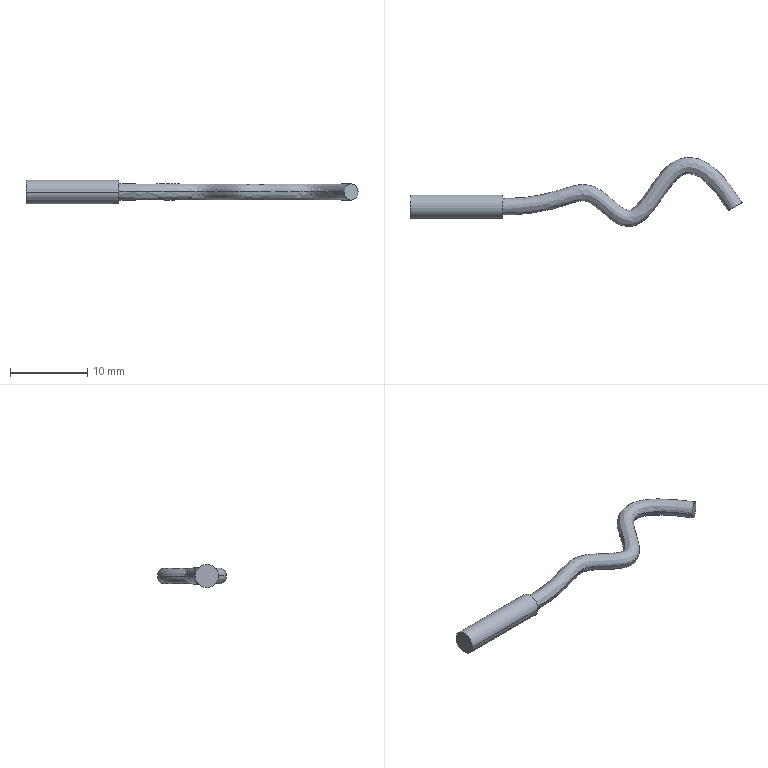Part | NX | 1 solid | 7 faces | box 42.898 x 8.936 x 3 mm | volume 211.409 mm3 | plane 3 | cylinder 2 | spline 2 | commonest cylinder face diameters 3 x2